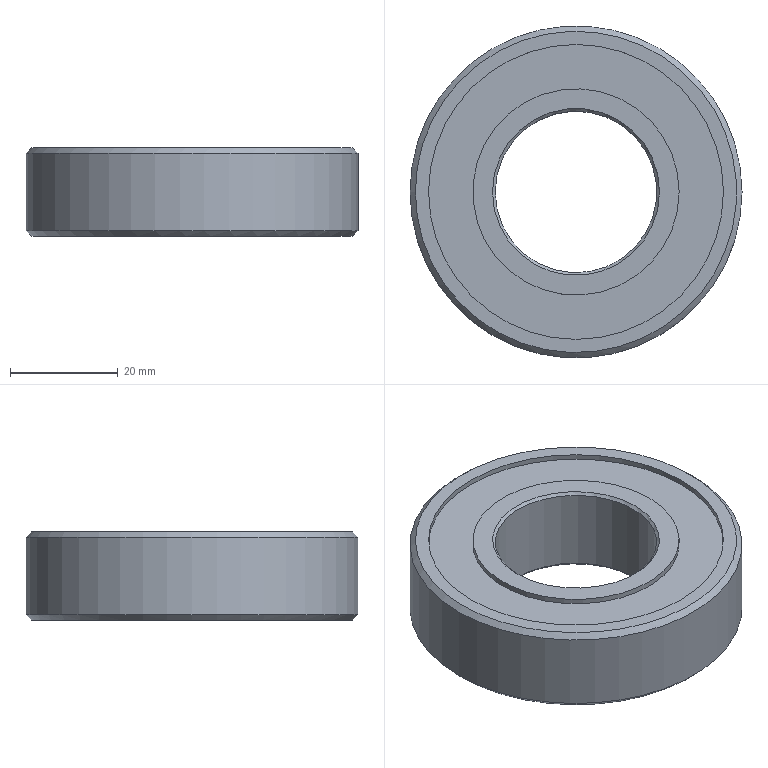Part | NX | features CHAMFER 4, DATUM_CSYS 4, EXTRUDE 3, SKETCH 3, DATUM_PLANE 2 | 1 solid | 16 faces | box 61.62 x 61.62 x 16.4 mm | volume 34698 mm3 | plane 6 | cylinder 6 | cone 4 | commonest cylinder face diameters 38.28 x2 54.72 x2 30 x1 61.62 x1
STEP:
#1=CARTESIAN_POINT('',(-15.5,0.,0.));
#2=VERTEX_POINT('',#1);
#3=CARTESIAN_POINT('',(0.,0.,0.));
#4=DIRECTION('',(0.,0.,-1.));
#5=DIRECTION('',(-1.,0.,0.));
#6=AXIS2_PLACEMENT_3D('',#3,#4,#5);
#7=CIRCLE('',#6,15.5);
#8=EDGE_CURVE('',#2,#2,#7,.F.);
#9=ORIENTED_EDGE('',*,*,#8,.T.);
#10=EDGE_LOOP('',(#9));
#11=FACE_BOUND('',#10,.T.);
#12=CARTESIAN_POINT('',(19.14,0.,0.));
#13=VERTEX_POINT('',#12);
#14=CARTESIAN_POINT('',(0.,0.,0.));
#15=DIRECTION('',(0.,0.,1.));
#16=DIRECTION('',(1.,0.,0.));
#17=AXIS2_PLACEMENT_3D('',#14,#15,#16);
#18=CIRCLE('',#17,19.14);
#19=EDGE_CURVE('',#13,#13,#18,.T.);
#20=ORIENTED_EDGE('',*,*,#19,.F.);
#21=EDGE_LOOP('',(#20));
#22=FACE_BOUND('',#21,.T.);
#23=CARTESIAN_POINT('',(0.,0.,0.));
#24=DIRECTION('',(0.,0.,-1.));
#25=DIRECTION('',(-1.,0.,0.));
#26=AXIS2_PLACEMENT_3D('',#23,#24,#25);
#27=PLANE('',#26);
#28=ADVANCED_FACE('',(#11,#22),#27,.T.);
#29=CARTESIAN_POINT('',(-15.5,0.,16.4));
#30=VERTEX_POINT('',#29);
#31=CARTESIAN_POINT('',(0.,0.,16.4));
#32=DIRECTION('',(0.,0.,-1.));
#33=DIRECTION('',(-1.,0.,0.));
#34=AXIS2_PLACEMENT_3D('',#31,#32,#33);
#35=CIRCLE('',#34,15.5);
#36=EDGE_CURVE('',#30,#30,#35,.T.);
#37=ORIENTED_EDGE('',*,*,#36,.T.);
#38=EDGE_LOOP('',(#37));
#39=FACE_BOUND('',#38,.T.);
#40=CARTESIAN_POINT('',(19.14,0.,16.4));
#41=VERTEX_POINT('',#40);
#42=CARTESIAN_POINT('',(0.,0.,16.4));
#43=DIRECTION('',(0.,0.,-1.));
#44=DIRECTION('',(1.,0.,0.));
#45=AXIS2_PLACEMENT_3D('',#42,#43,#44);
#46=CIRCLE('',#45,19.14);
#47=EDGE_CURVE('',#41,#41,#46,.T.);
#48=ORIENTED_EDGE('',*,*,#47,.F.);
#49=EDGE_LOOP('',(#48));
#50=FACE_BOUND('',#49,.T.);
#51=CARTESIAN_POINT('',(0.,0.,16.4));
#52=DIRECTION('',(0.,0.,-1.));
#53=DIRECTION('',(-1.,0.,0.));
#54=AXIS2_PLACEMENT_3D('',#51,#52,#53);
#55=PLANE('',#54);
#56=ADVANCED_FACE('',(#39,#50),#55,.F.);
#57=CARTESIAN_POINT('',(-30.81,0.,1.));
#58=VERTEX_POINT('',#57);
#59=CARTESIAN_POINT('',(0.,0.,1.));
#60=DIRECTION('',(0.,0.,-1.));
#61=DIRECTION('',(-1.,0.,0.));
#62=AXIS2_PLACEMENT_3D('',#59,#60,#61);
#63=CIRCLE('',#62,30.81);
#64=EDGE_CURVE('',#58,#58,#63,.F.);
#65=ORIENTED_EDGE('',*,*,#64,.T.);
#66=EDGE_LOOP('',(#65));
#67=FACE_BOUND('',#66,.T.);
#68=CARTESIAN_POINT('',(-30.81,0.,15.4));
#69=VERTEX_POINT('',#68);
#70=CARTESIAN_POINT('',(0.,0.,15.4));
#71=DIRECTION('',(0.,0.,-1.));
#72=DIRECTION('',(-1.,0.,0.));
#73=AXIS2_PLACEMENT_3D('',#70,#71,#72);
#74=CIRCLE('',#73,30.81);
#75=EDGE_CURVE('',#69,#69,#74,.T.);
#76=ORIENTED_EDGE('',*,*,#75,.T.);
#77=EDGE_LOOP('',(#76));
#78=FACE_BOUND('',#77,.T.);
#79=CARTESIAN_POINT('',(0.,0.,16.4));
#80=DIRECTION('',(0.,0.,-1.));
#81=DIRECTION('',(-1.,0.,0.));
#82=AXIS2_PLACEMENT_3D('',#79,#80,#81);
#83=CYLINDRICAL_SURFACE('',#82,30.81);
#84=ADVANCED_FACE('',(#67,#78),#83,.T.);
#85=CARTESIAN_POINT('',(-15.,0.,15.9));
#86=VERTEX_POINT('',#85);
#87=CARTESIAN_POINT('',(0.,0.,15.9));
#88=DIRECTION('',(0.,0.,-1.));
#89=DIRECTION('',(-1.,0.,0.));
#90=AXIS2_PLACEMENT_3D('',#87,#88,#89);
#91=CIRCLE('',#90,15.);
#92=EDGE_CURVE('',#86,#86,#91,.F.);
#93=ORIENTED_EDGE('',*,*,#92,.T.);
#94=EDGE_LOOP('',(#93));
#95=FACE_BOUND('',#94,.T.);
#96=CARTESIAN_POINT('',(-15.,0.,0.5));
#97=VERTEX_POINT('',#96);
#98=CARTESIAN_POINT('',(0.,0.,0.5));
#99=DIRECTION('',(0.,0.,-1.));
#100=DIRECTION('',(-1.,0.,0.));
#101=AXIS2_PLACEMENT_3D('',#98,#99,#100);
#102=CIRCLE('',#101,15.);
#103=EDGE_CURVE('',#97,#97,#102,.T.);
#104=ORIENTED_EDGE('',*,*,#103,.T.);
#105=EDGE_LOOP('',(#104));
#106=FACE_BOUND('',#105,.T.);
#107=CARTESIAN_POINT('',(0.,0.,16.4));
#108=DIRECTION('',(0.,0.,-1.));
#109=DIRECTION('',(-1.,0.,0.));
#110=AXIS2_PLACEMENT_3D('',#107,#108,#109);
#111=CYLINDRICAL_SURFACE('',#110,15.);
#112=ADVANCED_FACE('',(#95,#106),#111,.F.);
#113=CARTESIAN_POINT('',(-29.81,0.,16.4));
#114=VERTEX_POINT('',#113);
#115=CARTESIAN_POINT('',(0.,0.,16.4));
#116=DIRECTION('',(0.,0.,-1.));
#117=DIRECTION('',(-1.,0.,0.));
#118=AXIS2_PLACEMENT_3D('',#115,#116,#117);
#119=CIRCLE('',#118,29.81);
#120=EDGE_CURVE('',#114,#114,#119,.F.);
#121=ORIENTED_EDGE('',*,*,#120,.T.);
#122=EDGE_LOOP('',(#121));
#123=FACE_BOUND('',#122,.T.);
#124=CARTESIAN_POINT('',(27.36,0.,16.4));
#125=VERTEX_POINT('',#124);
#126=CARTESIAN_POINT('',(0.,0.,16.4));
#127=DIRECTION('',(0.,0.,-1.));
#128=DIRECTION('',(1.,0.,0.));
#129=AXIS2_PLACEMENT_3D('',#126,#127,#128);
#130=CIRCLE('',#129,27.36);
#131=EDGE_CURVE('',#125,#125,#130,.T.);
#132=ORIENTED_EDGE('',*,*,#131,.T.);
#133=EDGE_LOOP('',(#132));
#134=FACE_BOUND('',#133,.T.);
#135=CARTESIAN_POINT('',(0.,0.,16.4));
#136=DIRECTION('',(0.,0.,-1.));
#137=DIRECTION('',(-1.,0.,0.));
#138=AXIS2_PLACEMENT_3D('',#135,#136,#137);
#139=PLANE('',#138);
#140=ADVANCED_FACE('',(#123,#134),#139,.F.);
#141=CARTESIAN_POINT('',(-29.81,0.,0.));
#142=VERTEX_POINT('',#141);
#143=CARTESIAN_POINT('',(0.,0.,0.));
#144=DIRECTION('',(0.,0.,-1.));
#145=DIRECTION('',(-1.,0.,0.));
#146=AXIS2_PLACEMENT_3D('',#143,#144,#145);
#147=CIRCLE('',#146,29.81);
#148=EDGE_CURVE('',#142,#142,#147,.T.);
#149=ORIENTED_EDGE('',*,*,#148,.T.);
#150=EDGE_LOOP('',(#149));
#151=FACE_BOUND('',#150,.T.);
#152=CARTESIAN_POINT('',(27.36,0.,0.));
#153=VERTEX_POINT('',#152);
#154=CARTESIAN_POINT('',(0.,0.,0.));
#155=DIRECTION('',(0.,0.,1.));
#156=DIRECTION('',(1.,0.,0.));
#157=AXIS2_PLACEMENT_3D('',#154,#155,#156);
#158=CIRCLE('',#157,27.36);
#159=EDGE_CURVE('',#153,#153,#158,.T.);
#160=ORIENTED_EDGE('',*,*,#159,.T.);
#161=EDGE_LOOP('',(#160));
#162=FACE_BOUND('',#161,.T.);
#163=CARTESIAN_POINT('',(0.,0.,0.));
#164=DIRECTION('',(0.,0.,-1.));
#165=DIRECTION('',(-1.,0.,0.));
#166=AXIS2_PLACEMENT_3D('',#163,#164,#165);
#167=PLANE('',#166);
#168=ADVANCED_FACE('',(#151,#162),#167,.T.);
#169=CARTESIAN_POINT('',(27.36,0.,15.4));
#170=VERTEX_POINT('',#169);
#171=CARTESIAN_POINT('',(0.,0.,15.4));
#172=DIRECTION('',(0.,0.,-1.));
#173=DIRECTION('',(1.,0.,0.));
#174=AXIS2_PLACEMENT_3D('',#171,#172,#173);
#175=CIRCLE('',#174,27.36);
#176=EDGE_CURVE('',#170,#170,#175,.F.);
#177=ORIENTED_EDGE('',*,*,#176,.F.);
#178=EDGE_LOOP('',(#177));
#179=FACE_BOUND('',#178,.T.);
#180=ORIENTED_EDGE('',*,*,#131,.F.);
#181=EDGE_LOOP('',(#180));
#182=FACE_BOUND('',#181,.T.);
#183=CARTESIAN_POINT('',(0.,0.,15.4));
#184=DIRECTION('',(0.,0.,1.));
#185=DIRECTION('',(1.,0.,0.));
#186=AXIS2_PLACEMENT_3D('',#183,#184,#185);
#187=CYLINDRICAL_SURFACE('',#186,27.36);
#188=ADVANCED_FACE('',(#179,#182),#187,.F.);
#189=CARTESIAN_POINT('',(19.14,0.,15.4));
#190=VERTEX_POINT('',#189);
#191=CARTESIAN_POINT('',(0.,0.,15.4));
#192=DIRECTION('',(0.,0.,-1.));
#193=DIRECTION('',(1.,0.,0.));
#194=AXIS2_PLACEMENT_3D('',#191,#192,#193);
#195=CIRCLE('',#194,19.14);
#196=EDGE_CURVE('',#190,#190,#195,.F.);
#197=ORIENTED_EDGE('',*,*,#196,.T.);
#198=EDGE_LOOP('',(#197));
#199=FACE_BOUND('',#198,.T.);
#200=ORIENTED_EDGE('',*,*,#47,.T.);
#201=EDGE_LOOP('',(#200));
#202=FACE_BOUND('',#201,.T.);
#203=CARTESIAN_POINT('',(0.,0.,15.4));
#204=DIRECTION('',(0.,0.,1.));
#205=DIRECTION('',(1.,0.,0.));
#206=AXIS2_PLACEMENT_3D('',#203,#204,#205);
#207=CYLINDRICAL_SURFACE('',#206,19.14);
#208=ADVANCED_FACE('',(#199,#202),#207,.T.);
#209=ORIENTED_EDGE('',*,*,#176,.T.);
#210=EDGE_LOOP('',(#209));
#211=FACE_BOUND('',#210,.T.);
#212=ORIENTED_EDGE('',*,*,#196,.F.);
#213=EDGE_LOOP('',(#212));
#214=FACE_BOUND('',#213,.T.);
#215=CARTESIAN_POINT('',(0.,0.,15.4));
#216=DIRECTION('',(0.,0.,-1.));
#217=DIRECTION('',(-1.,0.,0.));
#218=AXIS2_PLACEMENT_3D('',#215,#216,#217);
#219=PLANE('',#218);
#220=ADVANCED_FACE('',(#211,#214),#219,.F.);
#221=CARTESIAN_POINT('',(27.36,0.,1.));
#222=VERTEX_POINT('',#221);
#223=CARTESIAN_POINT('',(0.,0.,1.));
#224=DIRECTION('',(0.,0.,1.));
#225=DIRECTION('',(1.,0.,0.));
#226=AXIS2_PLACEMENT_3D('',#223,#224,#225);
#227=CIRCLE('',#226,27.36);
#228=EDGE_CURVE('',#222,#222,#227,.F.);
#229=ORIENTED_EDGE('',*,*,#228,.F.);
#230=EDGE_LOOP('',(#229));
#231=FACE_BOUND('',#230,.T.);
#232=ORIENTED_EDGE('',*,*,#159,.F.);
#233=EDGE_LOOP('',(#232));
#234=FACE_BOUND('',#233,.T.);
#235=CARTESIAN_POINT('',(0.,0.,1.));
#236=DIRECTION('',(0.,0.,-1.));
#237=DIRECTION('',(-1.,0.,0.));
#238=AXIS2_PLACEMENT_3D('',#235,#236,#237);
#239=CYLINDRICAL_SURFACE('',#238,27.36);
#240=ADVANCED_FACE('',(#231,#234),#239,.F.);
#241=CARTESIAN_POINT('',(19.14,0.,1.));
#242=VERTEX_POINT('',#241);
#243=CARTESIAN_POINT('',(0.,0.,1.));
#244=DIRECTION('',(0.,0.,1.));
#245=DIRECTION('',(1.,0.,0.));
#246=AXIS2_PLACEMENT_3D('',#243,#244,#245);
#247=CIRCLE('',#246,19.14);
#248=EDGE_CURVE('',#242,#242,#247,.F.);
#249=ORIENTED_EDGE('',*,*,#248,.T.);
#250=EDGE_LOOP('',(#249));
#251=FACE_BOUND('',#250,.T.);
#252=ORIENTED_EDGE('',*,*,#19,.T.);
#253=EDGE_LOOP('',(#252));
#254=FACE_BOUND('',#253,.T.);
#255=CARTESIAN_POINT('',(0.,0.,1.));
#256=DIRECTION('',(0.,0.,-1.));
#257=DIRECTION('',(-1.,0.,0.));
#258=AXIS2_PLACEMENT_3D('',#255,#256,#257);
#259=CYLINDRICAL_SURFACE('',#258,19.14);
#260=ADVANCED_FACE('',(#251,#254),#259,.T.);
#261=ORIENTED_EDGE('',*,*,#228,.T.);
#262=EDGE_LOOP('',(#261));
#263=FACE_BOUND('',#262,.T.);
#264=ORIENTED_EDGE('',*,*,#248,.F.);
#265=EDGE_LOOP('',(#264));
#266=FACE_BOUND('',#265,.T.);
#267=CARTESIAN_POINT('',(0.,0.,1.));
#268=DIRECTION('',(0.,0.,1.));
#269=DIRECTION('',(1.,0.,0.));
#270=AXIS2_PLACEMENT_3D('',#267,#268,#269);
#271=PLANE('',#270);
#272=ADVANCED_FACE('',(#263,#266),#271,.F.);
#273=ORIENTED_EDGE('',*,*,#120,.F.);
#274=EDGE_LOOP('',(#273));
#275=FACE_BOUND('',#274,.T.);
#276=ORIENTED_EDGE('',*,*,#75,.F.);
#277=EDGE_LOOP('',(#276));
#278=FACE_BOUND('',#277,.T.);
#279=CARTESIAN_POINT('',(0.,0.,15.4));
#280=DIRECTION('',(0.,0.,-1.));
#281=DIRECTION('',(-1.,0.,0.));
#282=AXIS2_PLACEMENT_3D('',#279,#280,#281);
#283=CONICAL_SURFACE('',#282,30.81,0.7854);
#284=ADVANCED_FACE('',(#275,#278),#283,.T.);
#285=ORIENTED_EDGE('',*,*,#64,.F.);
#286=EDGE_LOOP('',(#285));
#287=FACE_BOUND('',#286,.T.);
#288=ORIENTED_EDGE('',*,*,#148,.F.);
#289=EDGE_LOOP('',(#288));
#290=FACE_BOUND('',#289,.T.);
#291=CARTESIAN_POINT('',(0.,0.,0.));
#292=DIRECTION('',(0.,0.,1.));
#293=DIRECTION('',(1.,0.,0.));
#294=AXIS2_PLACEMENT_3D('',#291,#292,#293);
#295=CONICAL_SURFACE('',#294,29.81,0.7854);
#296=ADVANCED_FACE('',(#287,#290),#295,.T.);
#297=ORIENTED_EDGE('',*,*,#8,.F.);
#298=EDGE_LOOP('',(#297));
#299=FACE_BOUND('',#298,.T.);
#300=ORIENTED_EDGE('',*,*,#103,.F.);
#301=EDGE_LOOP('',(#300));
#302=FACE_BOUND('',#301,.T.);
#303=CARTESIAN_POINT('',(0.,0.,0.5));
#304=DIRECTION('',(0.,0.,-1.));
#305=DIRECTION('',(-1.,0.,0.));
#306=AXIS2_PLACEMENT_3D('',#303,#304,#305);
#307=CONICAL_SURFACE('',#306,15.,0.7854);
#308=ADVANCED_FACE('',(#299,#302),#307,.F.);
#309=ORIENTED_EDGE('',*,*,#92,.F.);
#310=EDGE_LOOP('',(#309));
#311=FACE_BOUND('',#310,.T.);
#312=ORIENTED_EDGE('',*,*,#36,.F.);
#313=EDGE_LOOP('',(#312));
#314=FACE_BOUND('',#313,.T.);
#315=CARTESIAN_POINT('',(0.,0.,16.4));
#316=DIRECTION('',(0.,0.,1.));
#317=DIRECTION('',(1.,0.,0.));
#318=AXIS2_PLACEMENT_3D('',#315,#316,#317);
#319=CONICAL_SURFACE('',#318,15.5,0.7854);
#320=ADVANCED_FACE('',(#311,#314),#319,.F.);
#321=CLOSED_SHELL('',(#28,#56,#84,#112,#140,#168,#188,#208,#220,#240,#260,#272,#284,#296,#308,#320));
#322=MANIFOLD_SOLID_BREP('',#321);
#323=(LENGTH_UNIT()NAMED_UNIT(*)SI_UNIT(.MILLI.,.METRE.));
#324=UNCERTAINTY_MEASURE_WITH_UNIT(LENGTH_MEASURE(0.00001),#323,'','');
#325=(NAMED_UNIT(*)PLANE_ANGLE_UNIT()SI_UNIT($,.RADIAN.));
#326=(NAMED_UNIT(*)SI_UNIT($,.STERADIAN.)SOLID_ANGLE_UNIT());
#327=(GEOMETRIC_REPRESENTATION_CONTEXT(3)GLOBAL_UNCERTAINTY_ASSIGNED_CONTEXT((#324))GLOBAL_UNIT_ASSIGNED_CONTEXT((#323,#325,#326))REPRESENTATION_CONTEXT('',''));
#328=ADVANCED_BREP_SHAPE_REPRESENTATION('',(#322),#327);